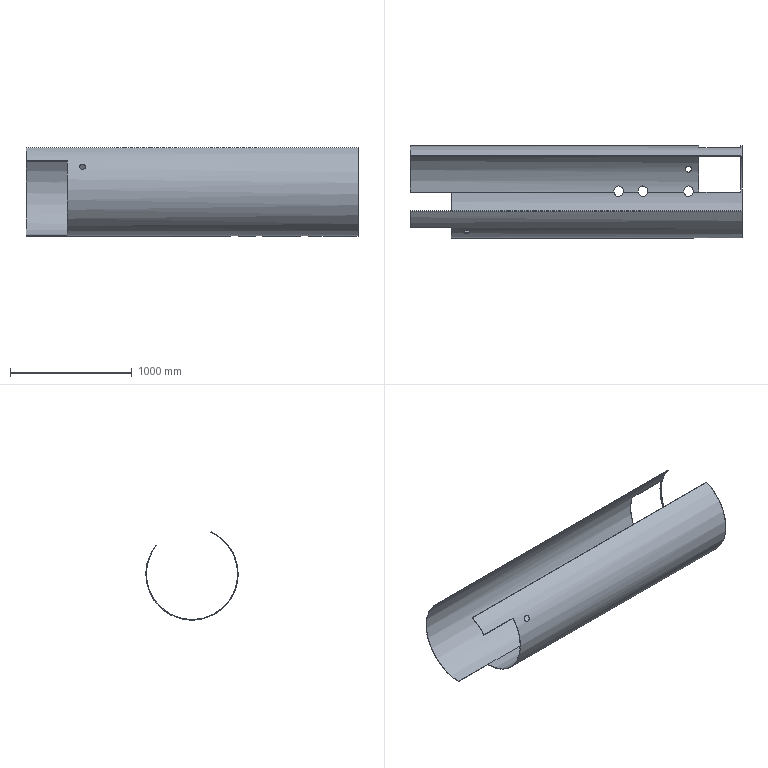Part | SolidWorks | features ICE 17, CirPattern 2, MirrorPattern 2, 3DProfileFeature 1, Extrusion 1, FlatPattern 1, FlattenBends 1, HoleWzd 1, ProcessBends 1, RefPoint 1, SheetMetal 1 | 1 solid | 28 faces | box 2730 x 759 x 724.83 mm | volume 18223877 mm3 | spline 12 | plane 12 | cylinder 4 | commonest cylinder face diameters 751 x2 759 x2